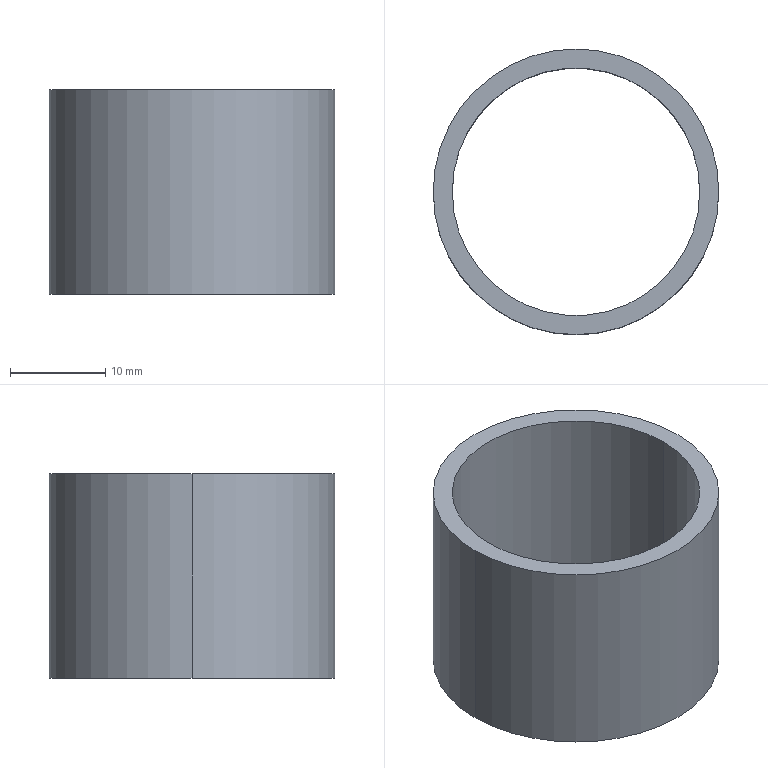Part | SolidWorks | features Extrusion 1 | 1 solid | 6 faces | box 30 x 30 x 21.5 mm | volume 3782 mm3 | cylinder 4 | plane 2 | commonest cylinder face diameters 26 x2 30 x2
STEP:
#1=CARTESIAN_POINT('',(-13.,0.,21.5));
#2=VERTEX_POINT('',#1);
#3=CARTESIAN_POINT('',(13.,0.,21.5));
#4=VERTEX_POINT('',#3);
#5=CARTESIAN_POINT('',(0.,0.,21.5));
#6=DIRECTION('',(0.,0.,1.));
#7=DIRECTION('',(1.,0.,0.));
#8=AXIS2_PLACEMENT_3D('',#5,#6,#7);
#9=CIRCLE('',#8,13.);
#10=EDGE_CURVE('',#2,#4,#9,.T.);
#11=ORIENTED_EDGE('',*,*,#10,.T.);
#12=CARTESIAN_POINT('',(13.,0.,0.));
#13=VERTEX_POINT('',#12);
#14=CARTESIAN_POINT('',(13.,0.,21.5));
#15=DIRECTION('',(0.,0.,-1.));
#16=VECTOR('',#15,1000.);
#17=LINE('',#14,#16);
#18=EDGE_CURVE('',#4,#13,#17,.T.);
#19=ORIENTED_EDGE('',*,*,#18,.T.);
#20=CARTESIAN_POINT('',(-13.,0.,0.));
#21=VERTEX_POINT('',#20);
#22=CARTESIAN_POINT('',(0.,0.,0.));
#23=DIRECTION('',(0.,0.,1.));
#24=DIRECTION('',(1.,0.,0.));
#25=AXIS2_PLACEMENT_3D('',#22,#23,#24);
#26=CIRCLE('',#25,13.);
#27=EDGE_CURVE('',#21,#13,#26,.T.);
#28=ORIENTED_EDGE('',*,*,#27,.F.);
#29=CARTESIAN_POINT('',(-13.,0.,21.5));
#30=DIRECTION('',(0.,0.,-1.));
#31=VECTOR('',#30,1000.);
#32=LINE('',#29,#31);
#33=EDGE_CURVE('',#2,#21,#32,.T.);
#34=ORIENTED_EDGE('',*,*,#33,.F.);
#35=EDGE_LOOP('',(#11,#19,#28,#34));
#36=FACE_OUTER_BOUND('',#35,.T.);
#37=CARTESIAN_POINT('',(0.,0.,21.5));
#38=DIRECTION('',(0.,0.,-1.));
#39=DIRECTION('',(-1.,0.,0.));
#40=AXIS2_PLACEMENT_3D('',#37,#38,#39);
#41=CYLINDRICAL_SURFACE('',#40,13.);
#42=ADVANCED_FACE('',(#36),#41,.F.);
#43=CARTESIAN_POINT('',(15.,0.,21.5));
#44=VERTEX_POINT('',#43);
#45=CARTESIAN_POINT('',(-15.,0.,21.5));
#46=VERTEX_POINT('',#45);
#47=CARTESIAN_POINT('',(0.,0.,21.5));
#48=DIRECTION('',(0.,0.,1.));
#49=DIRECTION('',(1.,0.,0.));
#50=AXIS2_PLACEMENT_3D('',#47,#48,#49);
#51=CIRCLE('',#50,15.);
#52=EDGE_CURVE('',#44,#46,#51,.T.);
#53=ORIENTED_EDGE('',*,*,#52,.F.);
#54=CARTESIAN_POINT('',(15.,0.,0.));
#55=VERTEX_POINT('',#54);
#56=CARTESIAN_POINT('',(15.,0.,21.5));
#57=DIRECTION('',(0.,0.,-1.));
#58=VECTOR('',#57,1000.);
#59=LINE('',#56,#58);
#60=EDGE_CURVE('',#44,#55,#59,.T.);
#61=ORIENTED_EDGE('',*,*,#60,.T.);
#62=CARTESIAN_POINT('',(-15.,0.,0.));
#63=VERTEX_POINT('',#62);
#64=CARTESIAN_POINT('',(0.,0.,0.));
#65=DIRECTION('',(0.,0.,1.));
#66=DIRECTION('',(1.,0.,0.));
#67=AXIS2_PLACEMENT_3D('',#64,#65,#66);
#68=CIRCLE('',#67,15.);
#69=EDGE_CURVE('',#55,#63,#68,.T.);
#70=ORIENTED_EDGE('',*,*,#69,.T.);
#71=CARTESIAN_POINT('',(-15.,0.,21.5));
#72=DIRECTION('',(0.,0.,-1.));
#73=VECTOR('',#72,1000.);
#74=LINE('',#71,#73);
#75=EDGE_CURVE('',#46,#63,#74,.T.);
#76=ORIENTED_EDGE('',*,*,#75,.F.);
#77=EDGE_LOOP('',(#53,#61,#70,#76));
#78=FACE_OUTER_BOUND('',#77,.T.);
#79=CARTESIAN_POINT('',(0.,0.,21.5));
#80=DIRECTION('',(0.,0.,-1.));
#81=DIRECTION('',(-1.,0.,0.));
#82=AXIS2_PLACEMENT_3D('',#79,#80,#81);
#83=CYLINDRICAL_SURFACE('',#82,15.);
#84=ADVANCED_FACE('',(#78),#83,.T.);
#85=CARTESIAN_POINT('',(0.,0.,21.5));
#86=DIRECTION('',(0.,0.,1.));
#87=DIRECTION('',(1.,0.,0.));
#88=AXIS2_PLACEMENT_3D('',#85,#86,#87);
#89=CIRCLE('',#88,15.);
#90=EDGE_CURVE('',#46,#44,#89,.T.);
#91=ORIENTED_EDGE('',*,*,#90,.T.);
#92=ORIENTED_EDGE('',*,*,#52,.T.);
#93=EDGE_LOOP('',(#91,#92));
#94=FACE_OUTER_BOUND('',#93,.T.);
#95=ORIENTED_EDGE('',*,*,#10,.F.);
#96=CARTESIAN_POINT('',(0.,0.,21.5));
#97=DIRECTION('',(0.,0.,1.));
#98=DIRECTION('',(1.,0.,0.));
#99=AXIS2_PLACEMENT_3D('',#96,#97,#98);
#100=CIRCLE('',#99,13.);
#101=EDGE_CURVE('',#4,#2,#100,.T.);
#102=ORIENTED_EDGE('',*,*,#101,.F.);
#103=EDGE_LOOP('',(#95,#102));
#104=FACE_BOUND('',#103,.T.);
#105=CARTESIAN_POINT('',(0.,0.,21.5));
#106=DIRECTION('',(0.,0.,1.));
#107=DIRECTION('',(1.,0.,0.));
#108=AXIS2_PLACEMENT_3D('',#105,#106,#107);
#109=PLANE('',#108);
#110=ADVANCED_FACE('',(#94,#104),#109,.T.);
#111=CARTESIAN_POINT('',(0.,0.,0.));
#112=DIRECTION('',(0.,0.,1.));
#113=DIRECTION('',(1.,0.,0.));
#114=AXIS2_PLACEMENT_3D('',#111,#112,#113);
#115=CIRCLE('',#114,15.);
#116=EDGE_CURVE('',#63,#55,#115,.T.);
#117=ORIENTED_EDGE('',*,*,#116,.F.);
#118=ORIENTED_EDGE('',*,*,#69,.F.);
#119=EDGE_LOOP('',(#117,#118));
#120=FACE_OUTER_BOUND('',#119,.T.);
#121=ORIENTED_EDGE('',*,*,#27,.T.);
#122=CARTESIAN_POINT('',(0.,0.,0.));
#123=DIRECTION('',(0.,0.,1.));
#124=DIRECTION('',(1.,0.,0.));
#125=AXIS2_PLACEMENT_3D('',#122,#123,#124);
#126=CIRCLE('',#125,13.);
#127=EDGE_CURVE('',#13,#21,#126,.T.);
#128=ORIENTED_EDGE('',*,*,#127,.T.);
#129=EDGE_LOOP('',(#121,#128));
#130=FACE_BOUND('',#129,.T.);
#131=CARTESIAN_POINT('',(0.,0.,0.));
#132=DIRECTION('',(0.,0.,1.));
#133=DIRECTION('',(1.,0.,0.));
#134=AXIS2_PLACEMENT_3D('',#131,#132,#133);
#135=PLANE('',#134);
#136=ADVANCED_FACE('',(#120,#130),#135,.F.);
#137=ORIENTED_EDGE('',*,*,#60,.F.);
#138=ORIENTED_EDGE('',*,*,#90,.F.);
#139=ORIENTED_EDGE('',*,*,#75,.T.);
#140=ORIENTED_EDGE('',*,*,#116,.T.);
#141=EDGE_LOOP('',(#137,#138,#139,#140));
#142=FACE_OUTER_BOUND('',#141,.T.);
#143=CARTESIAN_POINT('',(0.,0.,21.5));
#144=DIRECTION('',(0.,0.,-1.));
#145=DIRECTION('',(-1.,0.,0.));
#146=AXIS2_PLACEMENT_3D('',#143,#144,#145);
#147=CYLINDRICAL_SURFACE('',#146,15.);
#148=ADVANCED_FACE('',(#142),#147,.T.);
#149=ORIENTED_EDGE('',*,*,#18,.F.);
#150=ORIENTED_EDGE('',*,*,#101,.T.);
#151=ORIENTED_EDGE('',*,*,#33,.T.);
#152=ORIENTED_EDGE('',*,*,#127,.F.);
#153=EDGE_LOOP('',(#149,#150,#151,#152));
#154=FACE_OUTER_BOUND('',#153,.T.);
#155=CARTESIAN_POINT('',(0.,0.,21.5));
#156=DIRECTION('',(0.,0.,-1.));
#157=DIRECTION('',(-1.,0.,0.));
#158=AXIS2_PLACEMENT_3D('',#155,#156,#157);
#159=CYLINDRICAL_SURFACE('',#158,13.);
#160=ADVANCED_FACE('',(#154),#159,.F.);
#161=CLOSED_SHELL('',(#42,#84,#110,#136,#148,#160));
#162=MANIFOLD_SOLID_BREP('',#161);
#163=CARTESIAN_POINT('',(0.,0.,0.));
#164=DIRECTION('',(0.,0.,1.));
#165=DIRECTION('',(1.,0.,0.));
#166=AXIS2_PLACEMENT_3D('',#163,#164,#165);
#167=(LENGTH_UNIT()NAMED_UNIT(*)SI_UNIT(.MILLI.,.METRE.));
#168=UNCERTAINTY_MEASURE_WITH_UNIT(LENGTH_MEASURE(0.00001),#167,'','');
#169=(NAMED_UNIT(*)PLANE_ANGLE_UNIT()SI_UNIT($,.RADIAN.));
#170=(NAMED_UNIT(*)SI_UNIT($,.STERADIAN.)SOLID_ANGLE_UNIT());
#171=(GEOMETRIC_REPRESENTATION_CONTEXT(3)GLOBAL_UNCERTAINTY_ASSIGNED_CONTEXT((#168))GLOBAL_UNIT_ASSIGNED_CONTEXT((#167,#169,#170))REPRESENTATION_CONTEXT('',''));
#172=ADVANCED_BREP_SHAPE_REPRESENTATION('',(#162,#166),#171);